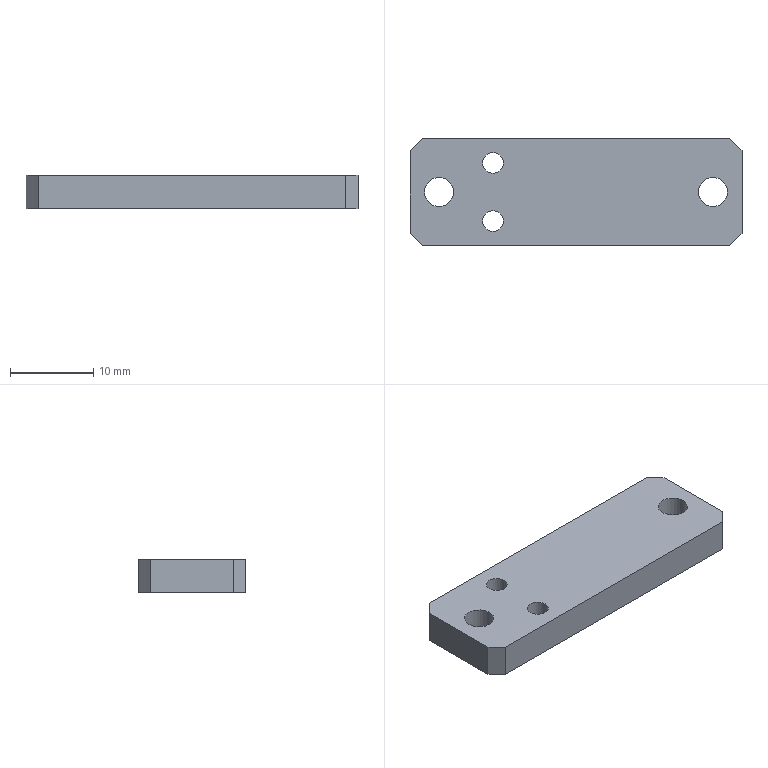Part | NX | 1 solid | 16 faces | box 40 x 13 x 4 mm | volume 1924 mm3 | plane 10 | cylinder 4 | cone 2 | commonest cylinder face diameters 2.5 x2 3.5 x2
STEP:
#1=CARTESIAN_POINT('',(20.,-5.,0.));
#2=VERTEX_POINT('',#1);
#3=CARTESIAN_POINT('',(20.,5.,0.));
#4=VERTEX_POINT('',#3);
#5=CARTESIAN_POINT('',(20.,-6.5,0.));
#6=DIRECTION('',(0.,1.,0.));
#7=VECTOR('',#6,1000.);
#8=LINE('',#5,#7);
#9=EDGE_CURVE('',#2,#4,#8,.T.);
#10=ORIENTED_EDGE('',*,*,#9,.T.);
#11=CARTESIAN_POINT('',(20.,5.,4.));
#12=VERTEX_POINT('',#11);
#13=CARTESIAN_POINT('',(20.,5.,4.));
#14=DIRECTION('',(0.,0.,1.));
#15=VECTOR('',#14,1000.);
#16=LINE('',#13,#15);
#17=EDGE_CURVE('',#4,#12,#16,.T.);
#18=ORIENTED_EDGE('',*,*,#17,.T.);
#19=CARTESIAN_POINT('',(20.,-5.,4.));
#20=VERTEX_POINT('',#19);
#21=CARTESIAN_POINT('',(20.,-6.5,4.));
#22=DIRECTION('',(0.,1.,0.));
#23=VECTOR('',#22,1000.);
#24=LINE('',#21,#23);
#25=EDGE_CURVE('',#20,#12,#24,.T.);
#26=ORIENTED_EDGE('',*,*,#25,.F.);
#27=CARTESIAN_POINT('',(20.,-5.,4.));
#28=DIRECTION('',(0.,0.,-1.));
#29=VECTOR('',#28,1000.);
#30=LINE('',#27,#29);
#31=EDGE_CURVE('',#20,#2,#30,.T.);
#32=ORIENTED_EDGE('',*,*,#31,.T.);
#33=EDGE_LOOP('',(#10,#18,#26,#32));
#34=FACE_BOUND('',#33,.T.);
#35=CARTESIAN_POINT('',(20.,-6.5,4.));
#36=DIRECTION('',(-1.,0.,0.));
#37=DIRECTION('',(0.,0.,1.));
#38=AXIS2_PLACEMENT_3D('',#35,#36,#37);
#39=PLANE('',#38);
#40=ADVANCED_FACE('',(#34),#39,.F.);
#41=CARTESIAN_POINT('',(18.5,6.5,4.));
#42=VERTEX_POINT('',#41);
#43=CARTESIAN_POINT('',(-18.5,6.5,4.));
#44=VERTEX_POINT('',#43);
#45=CARTESIAN_POINT('',(-20.,6.5,4.));
#46=DIRECTION('',(-1.,0.,0.));
#47=VECTOR('',#46,1000.);
#48=LINE('',#45,#47);
#49=EDGE_CURVE('',#42,#44,#48,.T.);
#50=ORIENTED_EDGE('',*,*,#49,.F.);
#51=CARTESIAN_POINT('',(18.5,6.5,0.));
#52=VERTEX_POINT('',#51);
#53=CARTESIAN_POINT('',(18.5,6.5,4.));
#54=DIRECTION('',(0.,0.,-1.));
#55=VECTOR('',#54,1000.);
#56=LINE('',#53,#55);
#57=EDGE_CURVE('',#42,#52,#56,.T.);
#58=ORIENTED_EDGE('',*,*,#57,.T.);
#59=CARTESIAN_POINT('',(-18.5,6.5,0.));
#60=VERTEX_POINT('',#59);
#61=CARTESIAN_POINT('',(-20.,6.5,0.));
#62=DIRECTION('',(-1.,0.,0.));
#63=VECTOR('',#62,1000.);
#64=LINE('',#61,#63);
#65=EDGE_CURVE('',#52,#60,#64,.T.);
#66=ORIENTED_EDGE('',*,*,#65,.T.);
#67=CARTESIAN_POINT('',(-18.5,6.5,4.));
#68=DIRECTION('',(0.,0.,1.));
#69=VECTOR('',#68,1000.);
#70=LINE('',#67,#69);
#71=EDGE_CURVE('',#60,#44,#70,.T.);
#72=ORIENTED_EDGE('',*,*,#71,.T.);
#73=EDGE_LOOP('',(#50,#58,#66,#72));
#74=FACE_BOUND('',#73,.T.);
#75=CARTESIAN_POINT('',(-20.,6.5,4.));
#76=DIRECTION('',(0.,-1.,0.));
#77=DIRECTION('',(0.,0.,-1.));
#78=AXIS2_PLACEMENT_3D('',#75,#76,#77);
#79=PLANE('',#78);
#80=ADVANCED_FACE('',(#74),#79,.F.);
#81=CARTESIAN_POINT('',(-20.,5.,0.));
#82=VERTEX_POINT('',#81);
#83=CARTESIAN_POINT('',(-20.,-5.,0.));
#84=VERTEX_POINT('',#83);
#85=CARTESIAN_POINT('',(-20.,-6.5,0.));
#86=DIRECTION('',(0.,-1.,0.));
#87=VECTOR('',#86,1000.);
#88=LINE('',#85,#87);
#89=EDGE_CURVE('',#82,#84,#88,.T.);
#90=ORIENTED_EDGE('',*,*,#89,.T.);
#91=CARTESIAN_POINT('',(-20.,-5.,4.));
#92=VERTEX_POINT('',#91);
#93=CARTESIAN_POINT('',(-20.,-5.,4.));
#94=DIRECTION('',(0.,0.,1.));
#95=VECTOR('',#94,1000.);
#96=LINE('',#93,#95);
#97=EDGE_CURVE('',#84,#92,#96,.T.);
#98=ORIENTED_EDGE('',*,*,#97,.T.);
#99=CARTESIAN_POINT('',(-20.,5.,4.));
#100=VERTEX_POINT('',#99);
#101=CARTESIAN_POINT('',(-20.,-6.5,4.));
#102=DIRECTION('',(0.,-1.,0.));
#103=VECTOR('',#102,1000.);
#104=LINE('',#101,#103);
#105=EDGE_CURVE('',#100,#92,#104,.T.);
#106=ORIENTED_EDGE('',*,*,#105,.F.);
#107=CARTESIAN_POINT('',(-20.,5.,4.));
#108=DIRECTION('',(0.,0.,-1.));
#109=VECTOR('',#108,1000.);
#110=LINE('',#107,#109);
#111=EDGE_CURVE('',#100,#82,#110,.T.);
#112=ORIENTED_EDGE('',*,*,#111,.T.);
#113=EDGE_LOOP('',(#90,#98,#106,#112));
#114=FACE_BOUND('',#113,.T.);
#115=CARTESIAN_POINT('',(-20.,-6.5,4.));
#116=DIRECTION('',(1.,0.,0.));
#117=DIRECTION('',(0.,0.,-1.));
#118=AXIS2_PLACEMENT_3D('',#115,#116,#117);
#119=PLANE('',#118);
#120=ADVANCED_FACE('',(#114),#119,.F.);
#121=CARTESIAN_POINT('',(-18.5,-6.5,0.));
#122=VERTEX_POINT('',#121);
#123=CARTESIAN_POINT('',(18.5,-6.5,0.));
#124=VERTEX_POINT('',#123);
#125=CARTESIAN_POINT('',(-20.,-6.5,0.));
#126=DIRECTION('',(1.,0.,0.));
#127=VECTOR('',#126,1000.);
#128=LINE('',#125,#127);
#129=EDGE_CURVE('',#122,#124,#128,.T.);
#130=ORIENTED_EDGE('',*,*,#129,.T.);
#131=CARTESIAN_POINT('',(18.5,-6.5,4.));
#132=VERTEX_POINT('',#131);
#133=CARTESIAN_POINT('',(18.5,-6.5,4.));
#134=DIRECTION('',(0.,0.,1.));
#135=VECTOR('',#134,1000.);
#136=LINE('',#133,#135);
#137=EDGE_CURVE('',#124,#132,#136,.T.);
#138=ORIENTED_EDGE('',*,*,#137,.T.);
#139=CARTESIAN_POINT('',(-18.5,-6.5,4.));
#140=VERTEX_POINT('',#139);
#141=CARTESIAN_POINT('',(-20.,-6.5,4.));
#142=DIRECTION('',(1.,0.,0.));
#143=VECTOR('',#142,1000.);
#144=LINE('',#141,#143);
#145=EDGE_CURVE('',#140,#132,#144,.T.);
#146=ORIENTED_EDGE('',*,*,#145,.F.);
#147=CARTESIAN_POINT('',(-18.5,-6.5,4.));
#148=DIRECTION('',(0.,0.,-1.));
#149=VECTOR('',#148,1000.);
#150=LINE('',#147,#149);
#151=EDGE_CURVE('',#140,#122,#150,.T.);
#152=ORIENTED_EDGE('',*,*,#151,.T.);
#153=EDGE_LOOP('',(#130,#138,#146,#152));
#154=FACE_BOUND('',#153,.T.);
#155=CARTESIAN_POINT('',(-20.,-6.5,4.));
#156=DIRECTION('',(0.,1.,0.));
#157=DIRECTION('',(0.,0.,1.));
#158=AXIS2_PLACEMENT_3D('',#155,#156,#157);
#159=PLANE('',#158);
#160=ADVANCED_FACE('',(#154),#159,.F.);
#161=CARTESIAN_POINT('',(-11.25,3.5,4.));
#162=VERTEX_POINT('',#161);
#163=CARTESIAN_POINT('',(-10.,3.5,4.));
#164=DIRECTION('',(0.,0.,-1.));
#165=DIRECTION('',(-1.,0.,0.));
#166=AXIS2_PLACEMENT_3D('',#163,#164,#165);
#167=CIRCLE('',#166,1.25);
#168=EDGE_CURVE('',#162,#162,#167,.T.);
#169=ORIENTED_EDGE('',*,*,#168,.T.);
#170=EDGE_LOOP('',(#169));
#171=FACE_BOUND('',#170,.T.);
#172=CARTESIAN_POINT('',(-11.25,-3.5,4.));
#173=VERTEX_POINT('',#172);
#174=CARTESIAN_POINT('',(-10.,-3.5,4.));
#175=DIRECTION('',(0.,0.,-1.));
#176=DIRECTION('',(-1.,0.,0.));
#177=AXIS2_PLACEMENT_3D('',#174,#175,#176);
#178=CIRCLE('',#177,1.25);
#179=EDGE_CURVE('',#173,#173,#178,.T.);
#180=ORIENTED_EDGE('',*,*,#179,.T.);
#181=EDGE_LOOP('',(#180));
#182=FACE_BOUND('',#181,.T.);
#183=CARTESIAN_POINT('',(14.75,0.,4.));
#184=VERTEX_POINT('',#183);
#185=CARTESIAN_POINT('',(16.5,0.,4.));
#186=DIRECTION('',(0.,0.,-1.));
#187=DIRECTION('',(-1.,0.,0.));
#188=AXIS2_PLACEMENT_3D('',#185,#186,#187);
#189=CIRCLE('',#188,1.75);
#190=EDGE_CURVE('',#184,#184,#189,.T.);
#191=ORIENTED_EDGE('',*,*,#190,.T.);
#192=EDGE_LOOP('',(#191));
#193=FACE_BOUND('',#192,.T.);
#194=CARTESIAN_POINT('',(-18.25,0.,4.));
#195=VERTEX_POINT('',#194);
#196=CARTESIAN_POINT('',(-16.5,0.,4.));
#197=DIRECTION('',(0.,0.,-1.));
#198=DIRECTION('',(-1.,0.,0.));
#199=AXIS2_PLACEMENT_3D('',#196,#197,#198);
#200=CIRCLE('',#199,1.75);
#201=EDGE_CURVE('',#195,#195,#200,.T.);
#202=ORIENTED_EDGE('',*,*,#201,.T.);
#203=EDGE_LOOP('',(#202));
#204=FACE_BOUND('',#203,.T.);
#205=ORIENTED_EDGE('',*,*,#25,.T.);
#206=CARTESIAN_POINT('',(18.5,6.5,4.));
#207=DIRECTION('',(0.7071,-0.7071,0.));
#208=VECTOR('',#207,1000.);
#209=LINE('',#206,#208);
#210=EDGE_CURVE('',#12,#42,#209,.F.);
#211=ORIENTED_EDGE('',*,*,#210,.T.);
#212=ORIENTED_EDGE('',*,*,#49,.T.);
#213=CARTESIAN_POINT('',(-20.,5.,4.));
#214=DIRECTION('',(0.7071,0.7071,0.));
#215=VECTOR('',#214,1000.);
#216=LINE('',#213,#215);
#217=EDGE_CURVE('',#44,#100,#216,.F.);
#218=ORIENTED_EDGE('',*,*,#217,.T.);
#219=ORIENTED_EDGE('',*,*,#105,.T.);
#220=CARTESIAN_POINT('',(-18.5,-6.5,4.));
#221=DIRECTION('',(-0.7071,0.7071,0.));
#222=VECTOR('',#221,1000.);
#223=LINE('',#220,#222);
#224=EDGE_CURVE('',#92,#140,#223,.F.);
#225=ORIENTED_EDGE('',*,*,#224,.T.);
#226=ORIENTED_EDGE('',*,*,#145,.T.);
#227=CARTESIAN_POINT('',(20.,-5.,4.));
#228=DIRECTION('',(-0.7071,-0.7071,0.));
#229=VECTOR('',#228,1000.);
#230=LINE('',#227,#229);
#231=EDGE_CURVE('',#132,#20,#230,.F.);
#232=ORIENTED_EDGE('',*,*,#231,.T.);
#233=EDGE_LOOP('',(#205,#211,#212,#218,#219,#225,#226,#232));
#234=FACE_BOUND('',#233,.T.);
#235=CARTESIAN_POINT('',(0.,0.,4.));
#236=DIRECTION('',(0.,0.,-1.));
#237=DIRECTION('',(-1.,0.,0.));
#238=AXIS2_PLACEMENT_3D('',#235,#236,#237);
#239=PLANE('',#238);
#240=ADVANCED_FACE('',(#171,#182,#193,#204,#234),#239,.F.);
#241=CARTESIAN_POINT('',(-11.25,3.5,0.));
#242=VERTEX_POINT('',#241);
#243=CARTESIAN_POINT('',(-10.,3.5,0.));
#244=DIRECTION('',(0.,0.,-1.));
#245=DIRECTION('',(-1.,0.,0.));
#246=AXIS2_PLACEMENT_3D('',#243,#244,#245);
#247=CIRCLE('',#246,1.25);
#248=EDGE_CURVE('',#242,#242,#247,.T.);
#249=ORIENTED_EDGE('',*,*,#248,.F.);
#250=EDGE_LOOP('',(#249));
#251=FACE_BOUND('',#250,.T.);
#252=CARTESIAN_POINT('',(-11.25,-3.5,0.));
#253=VERTEX_POINT('',#252);
#254=CARTESIAN_POINT('',(-10.,-3.5,0.));
#255=DIRECTION('',(0.,0.,-1.));
#256=DIRECTION('',(-1.,0.,0.));
#257=AXIS2_PLACEMENT_3D('',#254,#255,#256);
#258=CIRCLE('',#257,1.25);
#259=EDGE_CURVE('',#253,#253,#258,.T.);
#260=ORIENTED_EDGE('',*,*,#259,.F.);
#261=EDGE_LOOP('',(#260));
#262=FACE_BOUND('',#261,.T.);
#263=CARTESIAN_POINT('',(13.5,0.,0.));
#264=VERTEX_POINT('',#263);
#265=CARTESIAN_POINT('',(16.5,0.,0.));
#266=DIRECTION('',(0.,0.,-1.));
#267=DIRECTION('',(-1.,0.,0.));
#268=AXIS2_PLACEMENT_3D('',#265,#266,#267);
#269=CIRCLE('',#268,3.);
#270=EDGE_CURVE('',#264,#264,#269,.T.);
#271=ORIENTED_EDGE('',*,*,#270,.F.);
#272=EDGE_LOOP('',(#271));
#273=FACE_BOUND('',#272,.T.);
#274=CARTESIAN_POINT('',(-19.5,0.,0.));
#275=VERTEX_POINT('',#274);
#276=CARTESIAN_POINT('',(-16.5,0.,0.));
#277=DIRECTION('',(0.,0.,-1.));
#278=DIRECTION('',(-1.,0.,0.));
#279=AXIS2_PLACEMENT_3D('',#276,#277,#278);
#280=CIRCLE('',#279,3.);
#281=EDGE_CURVE('',#275,#275,#280,.T.);
#282=ORIENTED_EDGE('',*,*,#281,.F.);
#283=EDGE_LOOP('',(#282));
#284=FACE_BOUND('',#283,.T.);
#285=ORIENTED_EDGE('',*,*,#65,.F.);
#286=CARTESIAN_POINT('',(12.5,12.5,0.));
#287=DIRECTION('',(-0.7071,0.7071,0.));
#288=VECTOR('',#287,1000.);
#289=LINE('',#286,#288);
#290=EDGE_CURVE('',#52,#4,#289,.F.);
#291=ORIENTED_EDGE('',*,*,#290,.T.);
#292=ORIENTED_EDGE('',*,*,#9,.F.);
#293=CARTESIAN_POINT('',(12.5,-12.5,0.));
#294=DIRECTION('',(0.7071,0.7071,0.));
#295=VECTOR('',#294,1000.);
#296=LINE('',#293,#295);
#297=EDGE_CURVE('',#2,#124,#296,.F.);
#298=ORIENTED_EDGE('',*,*,#297,.T.);
#299=ORIENTED_EDGE('',*,*,#129,.F.);
#300=CARTESIAN_POINT('',(-12.5,-12.5,0.));
#301=DIRECTION('',(0.7071,-0.7071,0.));
#302=VECTOR('',#301,1000.);
#303=LINE('',#300,#302);
#304=EDGE_CURVE('',#122,#84,#303,.F.);
#305=ORIENTED_EDGE('',*,*,#304,.T.);
#306=ORIENTED_EDGE('',*,*,#89,.F.);
#307=CARTESIAN_POINT('',(-12.5,12.5,0.));
#308=DIRECTION('',(-0.7071,-0.7071,0.));
#309=VECTOR('',#308,1000.);
#310=LINE('',#307,#309);
#311=EDGE_CURVE('',#82,#60,#310,.F.);
#312=ORIENTED_EDGE('',*,*,#311,.T.);
#313=EDGE_LOOP('',(#285,#291,#292,#298,#299,#305,#306,#312));
#314=FACE_BOUND('',#313,.T.);
#315=CARTESIAN_POINT('',(0.,0.,0.));
#316=DIRECTION('',(0.,0.,-1.));
#317=DIRECTION('',(-1.,0.,0.));
#318=AXIS2_PLACEMENT_3D('',#315,#316,#317);
#319=PLANE('',#318);
#320=ADVANCED_FACE('',(#251,#262,#273,#284,#314),#319,.T.);
#321=ORIENTED_EDGE('',*,*,#210,.F.);
#322=ORIENTED_EDGE('',*,*,#17,.F.);
#323=ORIENTED_EDGE('',*,*,#290,.F.);
#324=ORIENTED_EDGE('',*,*,#57,.F.);
#325=EDGE_LOOP('',(#321,#322,#323,#324));
#326=FACE_BOUND('',#325,.T.);
#327=CARTESIAN_POINT('',(18.5,6.5,4.));
#328=DIRECTION('',(-0.7071,-0.7071,0.));
#329=DIRECTION('',(0.,0.,-1.));
#330=AXIS2_PLACEMENT_3D('',#327,#328,#329);
#331=PLANE('',#330);
#332=ADVANCED_FACE('',(#326),#331,.F.);
#333=ORIENTED_EDGE('',*,*,#231,.F.);
#334=ORIENTED_EDGE('',*,*,#137,.F.);
#335=ORIENTED_EDGE('',*,*,#297,.F.);
#336=ORIENTED_EDGE('',*,*,#31,.F.);
#337=EDGE_LOOP('',(#333,#334,#335,#336));
#338=FACE_BOUND('',#337,.T.);
#339=CARTESIAN_POINT('',(20.,-5.,4.));
#340=DIRECTION('',(-0.7071,0.7071,0.));
#341=DIRECTION('',(0.,0.,-1.));
#342=AXIS2_PLACEMENT_3D('',#339,#340,#341);
#343=PLANE('',#342);
#344=ADVANCED_FACE('',(#338),#343,.F.);
#345=ORIENTED_EDGE('',*,*,#224,.F.);
#346=ORIENTED_EDGE('',*,*,#97,.F.);
#347=ORIENTED_EDGE('',*,*,#304,.F.);
#348=ORIENTED_EDGE('',*,*,#151,.F.);
#349=EDGE_LOOP('',(#345,#346,#347,#348));
#350=FACE_BOUND('',#349,.T.);
#351=CARTESIAN_POINT('',(-18.5,-6.5,4.));
#352=DIRECTION('',(0.7071,0.7071,0.));
#353=DIRECTION('',(0.,0.,-1.));
#354=AXIS2_PLACEMENT_3D('',#351,#352,#353);
#355=PLANE('',#354);
#356=ADVANCED_FACE('',(#350),#355,.F.);
#357=ORIENTED_EDGE('',*,*,#217,.F.);
#358=ORIENTED_EDGE('',*,*,#71,.F.);
#359=ORIENTED_EDGE('',*,*,#311,.F.);
#360=ORIENTED_EDGE('',*,*,#111,.F.);
#361=EDGE_LOOP('',(#357,#358,#359,#360));
#362=FACE_BOUND('',#361,.T.);
#363=CARTESIAN_POINT('',(-20.,5.,4.));
#364=DIRECTION('',(0.7071,-0.7071,0.));
#365=DIRECTION('',(0.,0.,-1.));
#366=AXIS2_PLACEMENT_3D('',#363,#364,#365);
#367=PLANE('',#366);
#368=ADVANCED_FACE('',(#362),#367,.F.);
#369=ORIENTED_EDGE('',*,*,#201,.F.);
#370=EDGE_LOOP('',(#369));
#371=FACE_BOUND('',#370,.T.);
#372=CARTESIAN_POINT('',(-18.25,0.,1.25));
#373=VERTEX_POINT('',#372);
#374=CARTESIAN_POINT('',(-16.5,0.,1.25));
#375=DIRECTION('',(0.,0.,-1.));
#376=DIRECTION('',(-1.,0.,0.));
#377=AXIS2_PLACEMENT_3D('',#374,#375,#376);
#378=CIRCLE('',#377,1.75);
#379=EDGE_CURVE('',#373,#373,#378,.T.);
#380=ORIENTED_EDGE('',*,*,#379,.T.);
#381=EDGE_LOOP('',(#380));
#382=FACE_BOUND('',#381,.T.);
#383=CARTESIAN_POINT('',(-16.5,0.,0.));
#384=DIRECTION('',(0.,0.,-1.));
#385=DIRECTION('',(-1.,0.,0.));
#386=AXIS2_PLACEMENT_3D('',#383,#384,#385);
#387=CYLINDRICAL_SURFACE('',#386,1.75);
#388=ADVANCED_FACE('',(#371,#382),#387,.F.);
#389=ORIENTED_EDGE('',*,*,#379,.F.);
#390=EDGE_LOOP('',(#389));
#391=FACE_BOUND('',#390,.T.);
#392=ORIENTED_EDGE('',*,*,#281,.T.);
#393=EDGE_LOOP('',(#392));
#394=FACE_BOUND('',#393,.T.);
#395=CARTESIAN_POINT('',(-16.5,0.,0.));
#396=DIRECTION('',(0.,0.,-1.));
#397=DIRECTION('',(-1.,0.,0.));
#398=AXIS2_PLACEMENT_3D('',#395,#396,#397);
#399=CONICAL_SURFACE('',#398,3.,0.7854);
#400=ADVANCED_FACE('',(#391,#394),#399,.F.);
#401=ORIENTED_EDGE('',*,*,#190,.F.);
#402=EDGE_LOOP('',(#401));
#403=FACE_BOUND('',#402,.T.);
#404=CARTESIAN_POINT('',(14.75,0.,1.25));
#405=VERTEX_POINT('',#404);
#406=CARTESIAN_POINT('',(16.5,0.,1.25));
#407=DIRECTION('',(0.,0.,-1.));
#408=DIRECTION('',(-1.,0.,0.));
#409=AXIS2_PLACEMENT_3D('',#406,#407,#408);
#410=CIRCLE('',#409,1.75);
#411=EDGE_CURVE('',#405,#405,#410,.T.);
#412=ORIENTED_EDGE('',*,*,#411,.T.);
#413=EDGE_LOOP('',(#412));
#414=FACE_BOUND('',#413,.T.);
#415=CARTESIAN_POINT('',(16.5,0.,0.));
#416=DIRECTION('',(0.,0.,-1.));
#417=DIRECTION('',(-1.,0.,0.));
#418=AXIS2_PLACEMENT_3D('',#415,#416,#417);
#419=CYLINDRICAL_SURFACE('',#418,1.75);
#420=ADVANCED_FACE('',(#403,#414),#419,.F.);
#421=ORIENTED_EDGE('',*,*,#411,.F.);
#422=EDGE_LOOP('',(#421));
#423=FACE_BOUND('',#422,.T.);
#424=ORIENTED_EDGE('',*,*,#270,.T.);
#425=EDGE_LOOP('',(#424));
#426=FACE_BOUND('',#425,.T.);
#427=CARTESIAN_POINT('',(16.5,0.,0.));
#428=DIRECTION('',(0.,0.,-1.));
#429=DIRECTION('',(-1.,0.,0.));
#430=AXIS2_PLACEMENT_3D('',#427,#428,#429);
#431=CONICAL_SURFACE('',#430,3.,0.7854);
#432=ADVANCED_FACE('',(#423,#426),#431,.F.);
#433=ORIENTED_EDGE('',*,*,#179,.F.);
#434=EDGE_LOOP('',(#433));
#435=FACE_BOUND('',#434,.T.);
#436=ORIENTED_EDGE('',*,*,#259,.T.);
#437=EDGE_LOOP('',(#436));
#438=FACE_BOUND('',#437,.T.);
#439=CARTESIAN_POINT('',(-10.,-3.5,0.));
#440=DIRECTION('',(0.,0.,-1.));
#441=DIRECTION('',(-1.,0.,0.));
#442=AXIS2_PLACEMENT_3D('',#439,#440,#441);
#443=CYLINDRICAL_SURFACE('',#442,1.25);
#444=ADVANCED_FACE('',(#435,#438),#443,.F.);
#445=ORIENTED_EDGE('',*,*,#168,.F.);
#446=EDGE_LOOP('',(#445));
#447=FACE_BOUND('',#446,.T.);
#448=ORIENTED_EDGE('',*,*,#248,.T.);
#449=EDGE_LOOP('',(#448));
#450=FACE_BOUND('',#449,.T.);
#451=CARTESIAN_POINT('',(-10.,3.5,0.));
#452=DIRECTION('',(0.,0.,-1.));
#453=DIRECTION('',(-1.,0.,0.));
#454=AXIS2_PLACEMENT_3D('',#451,#452,#453);
#455=CYLINDRICAL_SURFACE('',#454,1.25);
#456=ADVANCED_FACE('',(#447,#450),#455,.F.);
#457=CLOSED_SHELL('',(#40,#80,#120,#160,#240,#320,#332,#344,#356,#368,#388,#400,#420,#432,#444,#456));
#458=MANIFOLD_SOLID_BREP('',#457);
#459=(LENGTH_UNIT()NAMED_UNIT(*)SI_UNIT(.MILLI.,.METRE.));
#460=UNCERTAINTY_MEASURE_WITH_UNIT(LENGTH_MEASURE(0.00001),#459,'','');
#461=(NAMED_UNIT(*)PLANE_ANGLE_UNIT()SI_UNIT($,.RADIAN.));
#462=(NAMED_UNIT(*)SI_UNIT($,.STERADIAN.)SOLID_ANGLE_UNIT());
#463=(GEOMETRIC_REPRESENTATION_CONTEXT(3)GLOBAL_UNCERTAINTY_ASSIGNED_CONTEXT((#460))GLOBAL_UNIT_ASSIGNED_CONTEXT((#459,#461,#462))REPRESENTATION_CONTEXT('',''));
#464=ADVANCED_BREP_SHAPE_REPRESENTATION('',(#458),#463);